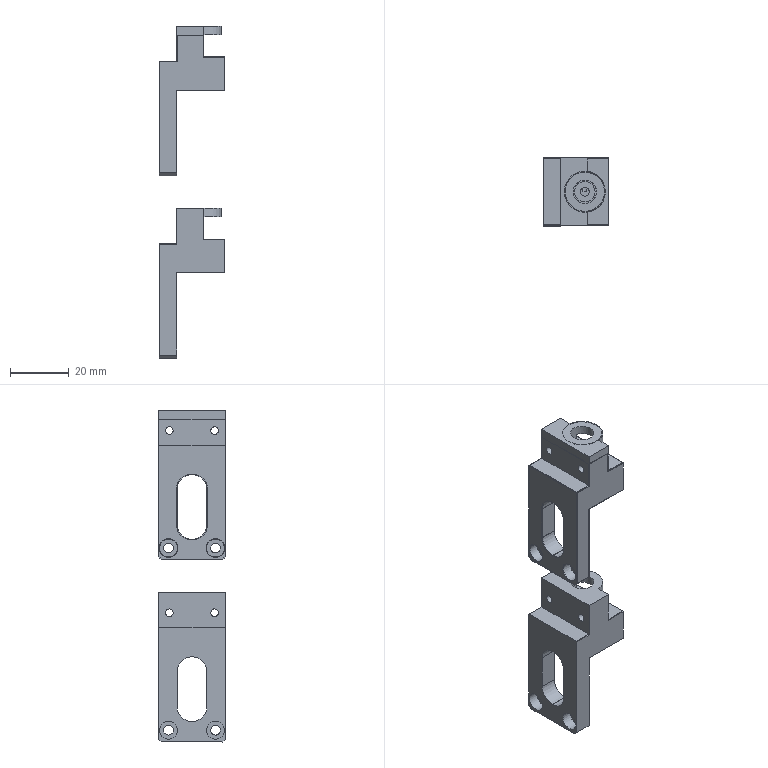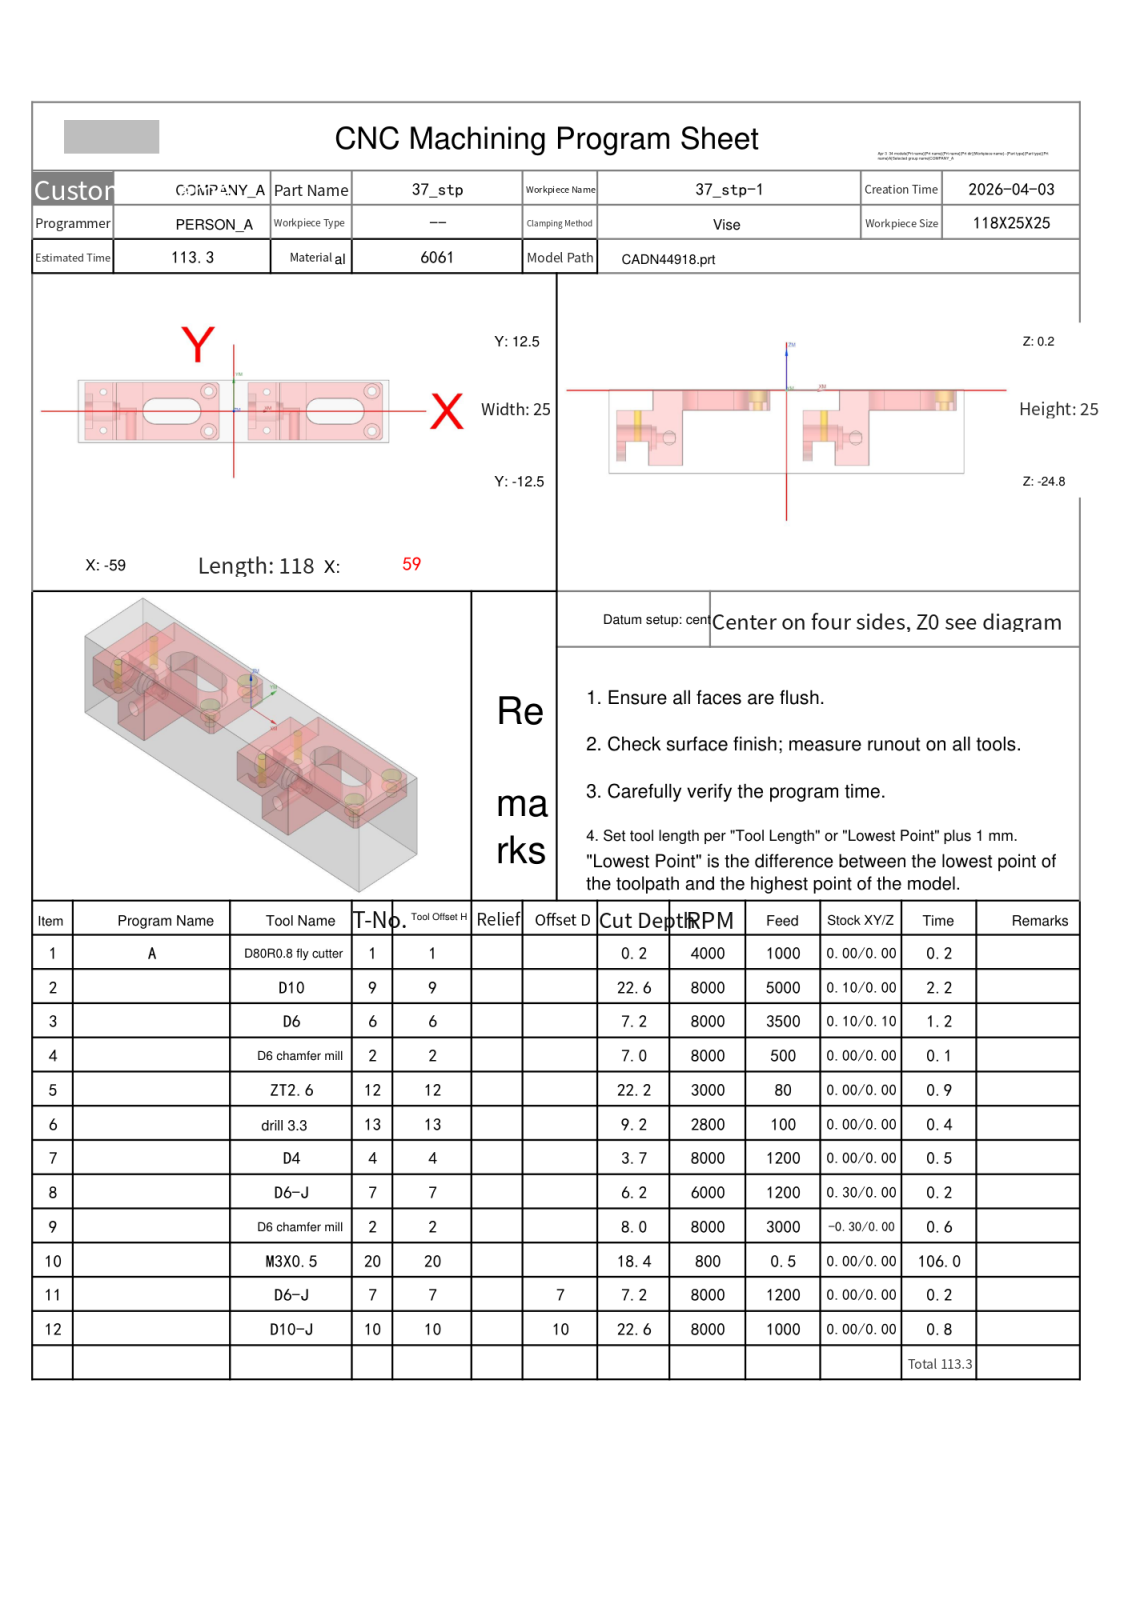NC program | NX | posted by the shop | part box 22.4 x 23 x 113 mm
Lines 1 to 2427 of 2531, first 1674 of 2425 lines:
%
O0001
(Machine time: 213.47 MIN)
(===Total Tool:10===)
(T1=D80R0.8 fly cutter D=80.  R=0.8  D-  H01 Z=0.    )
(T9=D10     D=10.  R=0.   D-  H09 Z=-22.4 )
(T6=D6      D=6.   R=0.   D-  H06 Z=-7.   )
(T2=D6 chamfer mill   D=6.   R=0.   D-  H02 Z=-7.8  )
(T12=ZT2.6  D=2.6  DR_a=118 D-  H12 Z=-22.  )
(T13=drill 3.3  D=3.3  DR_a=118 D-  H13 Z=-8.99 )
(T4=D4      D=4.   R=0.   D4  H04 Z=-3.5  )
(T7=D6-J    D=6.   R=0.   D-  H07 Z=-7.   )
(T20=M3X0.5 D=2.5  DR_a=180 D-  H20 Z=-18.25)
(T10=D10-J  D=10.  R=0.   D10 H10 Z=-22.4 )
G80 G90 G17 G49 G40
G91 G28 Z0
M01
N1 T01 M06
(D80R0.8 fly cutter  D=80. R=0.8 H=01 ce=0.00 di=0.00)
G00 G90 G54 X101.5 Y0.0 M03 S4000
G43 H01 Z20.
M08
Z2.
G01 Z0.0 F1000.
X96.5
X-96.5
X-101.5
Z2.
G00 Z20.
G91 G28 Z0.0
M05
M09
G91 G28 Z0.0
M01
N2 T09 M06
(D10  D=10. R=0. H=09 ce=0.10 di=0.00)
G00 G90 G54 X-31.5 Y-16.6 M03 S8000
G43 H09 Z20.
M08
Z.5
G01 X-56.5 Z.39 F5000.
G02 X-61.6 Y-11.5 Z.354 I0.0 J5.1
G01 Y11.5 Z.253
G02 X-56.5 Y16.6 Z.217 I5.1 J0.0
G01 X-45.75 Z.17
X-6.5 Z-.003
G02 X-2.894 Y15.106 Z-.021 I0.0 J-5.1
G01 X-1.894 Y14.106 Z-.027
G02 X-.4 Y10.5 Z-.045 I-3.606 J-3.606
G01 Y-10.5 Z-.138
G02 X-1.894 Y-14.106 Z-.155 I-5.1 J0.0
G01 X-2.894 Y-15.106 Z-.162
G02 X-6.5 Y-16.6 Z-.179 I-3.606 J3.606
G01 X-56.5 Z-.4
G02 X-61.6 Y-11.5 Z-.435 I0.0 J5.1
G01 Y11.5 Z-.537
G02 X-56.5 Y16.6 Z-.572 I5.1 J0.0
G01 X-45.75 Z-.62
X-6.5 Z-.793
G02 X-2.894 Y15.106 Z-.811 I0.0 J-5.1
G01 X-1.894 Y14.106 Z-.817
G02 X-.4 Y10.5 Z-.835 I-3.606 J-3.606
G01 Y-10.5 Z-.927
G02 X-1.894 Y-14.106 Z-.945 I-5.1 J0.0
G01 X-2.894 Y-15.106 Z-.951
G02 X-6.5 Y-16.6 Z-.969 I-3.606 J3.606
G01 X-56.5 Z-1.19
G02 X-61.6 Y-11.5 Z-1.225 I0.0 J5.1
G01 Y11.5 Z-1.327
G02 X-56.5 Y16.6 Z-1.362 I5.1 J0.0
G01 X-45.75 Z-1.409
X-6.5 Z-1.583
G02 X-2.894 Y15.106 Z-1.6 I0.0 J-5.1
G01 X-1.894 Y14.106 Z-1.607
G02 X-.4 Y10.5 Z-1.624 I-3.606 J-3.606
G01 Y-10.5 Z-1.717
G02 X-1.894 Y-14.106 Z-1.735 I-5.1 J0.0
G01 X-2.894 Y-15.106 Z-1.741
G02 X-6.5 Y-16.6 Z-1.759 I-3.606 J3.606
G01 X-56.5 Z-1.979
G02 X-61.6 Y-11.5 Z-2.015 I0.0 J5.1
G01 Y11.5 Z-2.116
G02 X-56.5 Y16.6 Z-2.152 I5.1 J0.0
G01 X-45.75 Z-2.199
X-6.5 Z-2.372
G02 X-2.894 Y15.106 Z-2.39 I0.0 J-5.1
G01 X-1.894 Y14.106 Z-2.396
G02 X-.4 Y10.5 Z-2.414 I-3.606 J-3.606
G01 Y-10.5 Z-2.507
G02 X-1.894 Y-14.106 Z-2.524 I-5.1 J0.0
G01 X-2.894 Y-15.106 Z-2.531
G02 X-6.5 Y-16.6 Z-2.548 I-3.606 J3.606
G01 X-56.5 Z-2.769
G02 X-61.6 Y-11.5 Z-2.804 I0.0 J5.1
G01 Y11.5 Z-2.906
G02 X-56.5 Y16.6 Z-2.941 I5.1 J0.0
G01 X-45.75 Z-2.989
X-6.5 Z-3.162
G02 X-2.894 Y15.106 Z-3.18 I0.0 J-5.1
G01 X-1.894 Y14.106 Z-3.186
G02 X-.4 Y10.5 Z-3.204 I-3.606 J-3.606
G01 Y-10.5 Z-3.296
G02 X-1.894 Y-14.106 Z-3.314 I-5.1 J0.0
G01 X-2.894 Y-15.106 Z-3.32
G02 X-6.5 Y-16.6 Z-3.338 I-3.606 J3.606
G01 X-56.5 Z-3.559
G02 X-61.6 Y-11.5 Z-3.594 I0.0 J5.1
G01 Y11.5 Z-3.696
G02 X-56.5 Y16.6 Z-3.731 I5.1 J0.0
G01 X-45.75 Z-3.778
X-6.5 Z-3.952
G02 X-2.894 Y15.106 Z-3.969 I0.0 J-5.1
G01 X-1.894 Y14.106 Z-3.976
G02 X-.4 Y10.5 Z-3.993 I-3.606 J-3.606
G01 Y-10.5 Z-4.086
G02 X-1.894 Y-14.106 Z-4.104 I-5.1 J0.0
G01 X-2.894 Y-15.106 Z-4.11
G02 X-6.5 Y-16.6 Z-4.128 I-3.606 J3.606
G01 X-56.5 Z-4.348
G02 X-61.6 Y-11.5 Z-4.384 I0.0 J5.1
G01 Y11.5 Z-4.485
G02 X-56.5 Y16.6 Z-4.521 I5.1 J0.0
G01 X-45.75 Z-4.568
X-6.5 Z-4.741
G02 X-2.894 Y15.106 Z-4.759 I0.0 J-5.1
G01 X-1.894 Y14.106 Z-4.765
G02 X-.4 Y10.5 Z-4.783 I-3.606 J-3.606
G01 Y-10.5 Z-4.876
G02 X-1.894 Y-14.106 Z-4.893 I-5.1 J0.0
G01 X-2.894 Y-15.106 Z-4.9
G02 X-6.5 Y-16.6 Z-4.917 I-3.606 J3.606
G01 X-56.5 Z-5.138
G02 X-61.6 Y-11.5 Z-5.173 I0.0 J5.1
G01 Y11.5 Z-5.275
G02 X-56.5 Y16.6 Z-5.31 I5.1 J0.0
G01 X-45.75 Z-5.358
X-6.5 Z-5.531
G02 X-2.894 Y15.106 Z-5.549 I0.0 J-5.1
G01 X-1.894 Y14.106 Z-5.555
G02 X-.4 Y10.5 Z-5.573 I-3.606 J-3.606
G01 Y-10.5 Z-5.665
G02 X-1.894 Y-14.106 Z-5.683 I-5.1 J0.0
G01 X-2.894 Y-15.106 Z-5.689
G02 X-6.5 Y-16.6 Z-5.707 I-3.606 J3.606
G01 X-56.5 Z-5.928
G02 X-61.6 Y-11.5 Z-5.963 I0.0 J5.1
G01 Y11.5 Z-6.065
G02 X-56.5 Y16.6 Z-6.1 I5.1 J0.0
G01 X-45.75 Z-6.147
X-6.5 Z-6.321
G02 X-2.894 Y15.106 Z-6.338 I0.0 J-5.1
G01 X-1.894 Y14.106 Z-6.345
G02 X-.4 Y10.5 Z-6.362 I-3.606 J-3.606
G01 Y-10.5 Z-6.455
G02 X-1.894 Y-14.106 Z-6.473 I-5.1 J0.0
G01 X-2.894 Y-15.106 Z-6.479
G02 X-6.5 Y-16.6 Z-6.497 I-3.606 J3.606
G01 X-56.5 Z-6.717
G02 X-61.6 Y-11.5 Z-6.753 I0.0 J5.1
G01 Y11.5 Z-6.854
G02 X-56.5 Y16.6 Z-6.89 I5.1 J0.0
G01 X-45.75 Z-6.937
X-6.5 Z-7.11
G02 X-2.894 Y15.106 Z-7.128 I0.0 J-5.1
G01 X-1.894 Y14.106 Z-7.134
G02 X-.4 Y10.5 Z-7.152 I-3.606 J-3.606
G01 Y-10.5 Z-7.245
G02 X-1.894 Y-14.106 Z-7.262 I-5.1 J0.0
G01 X-2.894 Y-15.106 Z-7.269
G02 X-6.5 Y-16.6 Z-7.286 I-3.606 J3.606
G01 X-56.5 Z-7.507
G02 X-61.6 Y-11.5 Z-7.542 I0.0 J5.1
G01 Y11.5 Z-7.644
G02 X-56.5 Y16.6 Z-7.679 I5.1 J0.0
G01 X-45.75 Z-7.727
X-6.5 Z-7.9
G02 X-2.894 Y15.106 Z-7.918 I0.0 J-5.1
G01 X-1.894 Y14.106 Z-7.924
G02 X-.4 Y10.5 Z-7.942 I-3.606 J-3.606
G01 Y-10.5 Z-8.034
G02 X-1.894 Y-14.106 Z-8.052 I-5.1 J0.0
G01 X-2.894 Y-15.106 Z-8.058
G02 X-6.5 Y-16.6 Z-8.076 I-3.606 J3.606
G01 X-56.5 Z-8.297
G02 X-61.6 Y-11.5 Z-8.332 I0.0 J5.1
G01 Y11.5 Z-8.433
G02 X-56.5 Y16.6 Z-8.469 I5.1 J0.0
G01 X-45.75 Z-8.516
X-6.5 Z-8.69
G02 X-2.894 Y15.106 Z-8.707 I0.0 J-5.1
G01 X-1.894 Y14.106 Z-8.713
G02 X-.4 Y10.5 Z-8.731 I-3.606 J-3.606
G01 Y-10.5 Z-8.824
G02 X-1.894 Y-14.106 Z-8.842 I-5.1 J0.0
G01 X-2.894 Y-15.106 Z-8.848
G02 X-6.5 Y-16.6 Z-8.865 I-3.606 J3.606
G01 X-56.5 Z-9.086
G02 X-61.6 Y-11.5 Z-9.122 I0.0 J5.1
G01 Y11.5 Z-9.223
G02 X-56.5 Y16.6 Z-9.258 I5.1 J0.0
G01 X-45.75 Z-9.306
X-6.5 Z-9.479
G02 X-2.894 Y15.106 Z-9.497 I0.0 J-5.1
G01 X-1.894 Y14.106 Z-9.503
G02 X-.4 Y10.5 Z-9.521 I-3.606 J-3.606
G01 Y-10.5 Z-9.614
G02 X-1.894 Y-14.106 Z-9.631 I-5.1 J0.0
G01 X-2.894 Y-15.106 Z-9.637
G02 X-6.5 Y-16.6 Z-9.655 I-3.606 J3.606
G01 X-56.5 Z-9.876
G02 X-61.6 Y-11.5 Z-9.911 I0.0 J5.1
G01 Y11.5 Z-10.013
G02 X-56.5 Y16.6 Z-10.048 I5.1 J0.0
G01 X-45.75 Z-10.096
X-6.5 Z-10.269
G02 X-2.894 Y15.106 Z-10.287 I0.0 J-5.1
G01 X-1.894 Y14.106 Z-10.293
G02 X-.4 Y10.5 Z-10.31 I-3.606 J-3.606
G01 Y-10.5 Z-10.403
G02 X-1.894 Y-14.106 Z-10.421 I-5.1 J0.0
G01 X-2.894 Y-15.106 Z-10.427
G02 X-6.5 Y-16.6 Z-10.445 I-3.606 J3.606
G01 X-56.5 Z-10.666
G02 X-61.6 Y-11.5 Z-10.701 I0.0 J5.1
G01 Y11.5 Z-10.802
G02 X-56.5 Y16.6 Z-10.838 I5.1 J0.0
G01 X-45.75 Z-10.885
X-6.5 Z-11.059
G02 X-2.894 Y15.106 Z-11.076 I0.0 J-5.1
G01 X-1.894 Y14.106 Z-11.082
G02 X-.4 Y10.5 Z-11.1 I-3.606 J-3.606
G01 Y-10.5 Z-11.193
G02 X-1.894 Y-14.106 Z-11.211 I-5.1 J0.0
G01 X-2.894 Y-15.106 Z-11.217
G02 X-6.5 Y-16.6 Z-11.234 I-3.606 J3.606
G01 X-56.5 Z-11.455
G02 X-61.6 Y-11.5 Z-11.491 I0.0 J5.1
G01 Y11.5 Z-11.592
G02 X-56.5 Y16.6 Z-11.627 I5.1 J0.0
G01 X-45.75 Z-11.675
X-6.5 Z-11.848
G02 X-2.894 Y15.106 Z-11.866 I0.0 J-5.1
G01 X-1.894 Y14.106 Z-11.872
G02 X-.4 Y10.5 Z-11.89 I-3.606 J-3.606
G01 Y-10.5 Z-11.983
G02 X-1.894 Y-14.106 Z-12. I-5.1 J0.0
G01 X-2.894 Y-15.106 Z-12.006
G02 X-6.5 Y-16.6 Z-12.024 I-3.606 J3.606
G01 X-56.5 Z-12.245
G02 X-61.6 Y-11.5 Z-12.28 I0.0 J5.1
G01 Y11.5 Z-12.382
G02 X-56.5 Y16.6 Z-12.417 I5.1 J0.0
G01 X-45.75 Z-12.465
X-6.5 Z-12.638
G02 X-2.894 Y15.106 Z-12.656 I0.0 J-5.1
G01 X-1.894 Y14.106 Z-12.662
G02 X-.4 Y10.5 Z-12.679 I-3.606 J-3.606
G01 Y-10.5 Z-12.772
G02 X-1.894 Y-14.106 Z-12.79 I-5.1 J0.0
G01 X-2.894 Y-15.106 Z-12.796
G02 X-6.5 Y-16.6 Z-12.814 I-3.606 J3.606
G01 X-56.5 Z-13.035
G02 X-61.6 Y-11.5 Z-13.07 I0.0 J5.1
G01 Y11.5 Z-13.171
G02 X-56.5 Y16.6 Z-13.207 I5.1 J0.0
G01 X-45.75 Z-13.254
X-6.5 Z-13.428
G02 X-2.894 Y15.106 Z-13.445 I0.0 J-5.1
G01 X-1.894 Y14.106 Z-13.451
G02 X-.4 Y10.5 Z-13.469 I-3.606 J-3.606
G01 Y-10.5 Z-13.562
G02 X-1.894 Y-14.106 Z-13.58 I-5.1 J0.0
G01 X-2.894 Y-15.106 Z-13.586
G02 X-6.5 Y-16.6 Z-13.603 I-3.606 J3.606
G01 X-56.5 Z-13.824
G02 X-61.6 Y-11.5 Z-13.86 I0.0 J5.1
G01 Y11.5 Z-13.961
G02 X-56.5 Y16.6 Z-13.996 I5.1 J0.0
G01 X-45.75 Z-14.044
X-6.5 Z-14.217
G02 X-2.894 Y15.106 Z-14.235 I0.0 J-5.1
G01 X-1.894 Y14.106 Z-14.241
G02 X-.4 Y10.5 Z-14.259 I-3.606 J-3.606
G01 Y-10.5 Z-14.351
G02 X-1.894 Y-14.106 Z-14.369 I-5.1 J0.0
G01 X-2.894 Y-15.106 Z-14.375
G02 X-6.5 Y-16.6 Z-14.393 I-3.606 J3.606
G01 X-56.5 Z-14.614
G02 X-61.6 Y-11.5 Z-14.649 I0.0 J5.1
G01 Y11.5 Z-14.751
G02 X-56.5 Y16.6 Z-14.786 I5.1 J0.0
G01 X-45.75 Z-14.834
X-6.5 Z-15.007
G02 X-2.894 Y15.106 Z-15.024 I0.0 J-5.1
G01 X-1.894 Y14.106 Z-15.031
G02 X-.4 Y10.5 Z-15.048 I-3.606 J-3.606
G01 Y-10.5 Z-15.141
G02 X-1.894 Y-14.106 Z-15.159 I-5.1 J0.0
G01 X-2.894 Y-15.106 Z-15.165
G02 X-6.5 Y-16.6 Z-15.183 I-3.606 J3.606
G01 X-56.5 Z-15.403
G02 X-61.6 Y-11.5 Z-15.439 I0.0 J5.1
G01 Y11.5 Z-15.54
G02 X-56.5 Y16.6 Z-15.576 I5.1 J0.0
G01 X-45.75 Z-15.623
X-6.5 Z-15.796
G02 X-2.894 Y15.106 Z-15.814 I0.0 J-5.1
G01 X-1.894 Y14.106 Z-15.82
G02 X-.4 Y10.5 Z-15.838 I-3.606 J-3.606
G01 Y-10.5 Z-15.931
G02 X-1.894 Y-14.106 Z-15.948 I-5.1 J0.0
G01 X-2.894 Y-15.106 Z-15.955
G02 X-6.5 Y-16.6 Z-15.972 I-3.606 J3.606
G01 X-56.5 Z-16.193
G02 X-61.6 Y-11.5 Z-16.228 I0.0 J5.1
G01 Y11.5 Z-16.33
G02 X-56.5 Y16.6 Z-16.365 I5.1 J0.0
G01 X-45.75 Z-16.413
X-6.5 Z-16.586
G02 X-2.894 Y15.106 Z-16.604 I0.0 J-5.1
G01 X-1.894 Y14.106 Z-16.61
G02 X-.4 Y10.5 Z-16.628 I-3.606 J-3.606
G01 Y-10.5 Z-16.72
G02 X-1.894 Y-14.106 Z-16.738 I-5.1 J0.0
G01 X-2.894 Y-15.106 Z-16.744
G02 X-6.5 Y-16.6 Z-16.762 I-3.606 J3.606
G01 X-56.5 Z-16.983
G02 X-61.6 Y-11.5 Z-17.018 I0.0 J5.1
G01 Y11.5 Z-17.12
G02 X-56.5 Y16.6 Z-17.155 I5.1 J0.0
G01 X-45.75 Z-17.203
X-6.5 Z-17.376
G02 X-2.894 Y15.106 Z-17.393 I0.0 J-5.1
G01 X-1.894 Y14.106 Z-17.4
G02 X-.4 Y10.5 Z-17.417 I-3.606 J-3.606
G01 Y-10.5 Z-17.51
G02 X-1.894 Y-14.106 Z-17.528 I-5.1 J0.0
G01 X-2.894 Y-15.106 Z-17.534
G02 X-6.5 Y-16.6 Z-17.552 I-3.606 J3.606
G01 X-56.5 Z-17.772
G02 X-61.6 Y-11.5 Z-17.808 I0.0 J5.1
G01 Y11.5 Z-17.909
G02 X-56.5 Y16.6 Z-17.945 I5.1 J0.0
G01 X-45.75 Z-17.992
X-6.5 Z-18.165
G02 X-2.894 Y15.106 Z-18.183 I0.0 J-5.1
G01 X-1.894 Y14.106 Z-18.189
G02 X-.4 Y10.5 Z-18.207 I-3.606 J-3.606
G01 Y-10.5 Z-18.3
G02 X-1.894 Y-14.106 Z-18.317 I-5.1 J0.0
G01 X-2.894 Y-15.106 Z-18.324
G02 X-6.5 Y-16.6 Z-18.341 I-3.606 J3.606
G01 X-56.5 Z-18.562
G02 X-61.6 Y-11.5 Z-18.597 I0.0 J5.1
G01 Y11.5 Z-18.699
G02 X-56.5 Y16.6 Z-18.734 I5.1 J0.0
G01 X-45.75 Z-18.782
X-6.5 Z-18.955
G02 X-2.894 Y15.106 Z-18.973 I0.0 J-5.1
G01 X-1.894 Y14.106 Z-18.979
G02 X-.4 Y10.5 Z-18.997 I-3.606 J-3.606
G01 Y-10.5 Z-19.089
G02 X-1.894 Y-14.106 Z-19.107 I-5.1 J0.0
G01 X-2.894 Y-15.106 Z-19.113
G02 X-6.5 Y-16.6 Z-19.131 I-3.606 J3.606
G01 X-56.5 Z-19.352
G02 X-61.6 Y-11.5 Z-19.387 I0.0 J5.1
G01 Y11.5 Z-19.489
G02 X-56.5 Y16.6 Z-19.524 I5.1 J0.0
G01 X-45.75 Z-19.571
X-6.5 Z-19.745
G02 X-2.894 Y15.106 Z-19.762 I0.0 J-5.1
G01 X-1.894 Y14.106 Z-19.769
G02 X-.4 Y10.5 Z-19.786 I-3.606 J-3.606
G01 Y-10.5 Z-19.879
G02 X-1.894 Y-14.106 Z-19.897 I-5.1 J0.0
G01 X-2.894 Y-15.106 Z-19.903
G02 X-6.5 Y-16.6 Z-19.921 I-3.606 J3.606
G01 X-56.5 Z-20.141
G02 X-61.6 Y-11.5 Z-20.177 I0.0 J5.1
G01 Y11.5 Z-20.278
G02 X-56.5 Y16.6 Z-20.314 I5.1 J0.0
G01 X-45.75 Z-20.361
X-6.5 Z-20.534
G02 X-2.894 Y15.106 Z-20.552 I0.0 J-5.1
G01 X-1.894 Y14.106 Z-20.558
G02 X-.4 Y10.5 Z-20.576 I-3.606 J-3.606
G01 Y-10.5 Z-20.669
G02 X-1.894 Y-14.106 Z-20.686 I-5.1 J0.0
G01 X-2.894 Y-15.106 Z-20.693
G02 X-6.5 Y-16.6 Z-20.71 I-3.606 J3.606
G01 X-56.5 Z-20.931
G02 X-61.6 Y-11.5 Z-20.966 I0.0 J5.1
G01 Y11.5 Z-21.068
G02 X-56.5 Y16.6 Z-21.103 I5.1 J0.0
G01 X-45.75 Z-21.151
X-6.5 Z-21.324
G02 X-2.894 Y15.106 Z-21.342 I0.0 J-5.1
G01 X-1.894 Y14.106 Z-21.348
G02 X-.4 Y10.5 Z-21.366 I-3.606 J-3.606
G01 Y-10.5 Z-21.458
G02 X-1.894 Y-14.106 Z-21.476 I-5.1 J0.0
G01 X-2.894 Y-15.106 Z-21.482
G02 X-6.5 Y-16.6 Z-21.5 I-3.606 J3.606
G01 X-56.5 Z-21.721
G02 X-61.6 Y-11.5 Z-21.756 I0.0 J5.1
G01 Y11.5 Z-21.858
G02 X-56.5 Y16.6 Z-21.893 I5.1 J0.0
G01 X-45.75 Z-21.94
X-6.5 Z-22.114
G02 X-2.894 Y15.106 Z-22.131 I0.0 J-5.1
G01 X-1.894 Y14.106 Z-22.138
G02 X-.4 Y10.5 Z-22.155 I-3.606 J-3.606
G01 Y-10.5 Z-22.248
G02 X-1.894 Y-14.106 Z-22.266 I-5.1 J0.0
G01 X-2.894 Y-15.106 Z-22.272
G02 X-6.5 Y-16.6 Z-22.29 I-3.606 J3.606
G01 X-31.5 Z-22.4
X-56.5
G02 X-61.6 Y-11.5 I0.0 J5.1
G01 Y11.5
G02 X-56.5 Y16.6 I5.1 J0.0
G01 X-45.75
X-6.5
G02 X-2.894 Y15.106 I0.0 J-5.1
G01 X-1.894 Y14.106
G02 X-.4 Y10.5 I-3.606 J-3.606
G01 Y-10.5
G02 X-1.894 Y-14.106 I-5.1 J0.0
G01 X-2.894 Y-15.106
G02 X-6.5 Y-16.6 I-3.606 J3.606
G01 X-31.5
X-32.
Z-21.4
G00 Z20.
X30.5
Z.5
G01 X5.5 Z.39
G02 X.4 Y-11.5 Z.354 I0.0 J5.1
G01 Y11.5 Z.253
G02 X3.44 Y16.165 Z.227 I5.1 J0.0
X5.5 Y16.6 Z.217 I2.06 J-4.665
G01 X55.5 Z-.003
G02 X59.106 Y15.106 Z-.021 I0.0 J-5.1
G01 X60.106 Y14.106 Z-.027
G02 X61.6 Y10.5 Z-.045 I-3.606 J-3.606
G01 Y-10.5 Z-.138
G02 X60.106 Y-14.106 Z-.155 I-5.1 J0.0
G01 X59.106 Y-15.106 Z-.162
G02 X55.5 Y-16.6 Z-.179 I-3.606 J3.606
G01 X5.5 Z-.4
G02 X.4 Y-11.5 Z-.435 I0.0 J5.1
G01 Y11.5 Z-.537
G02 X3.44 Y16.165 Z-.563 I5.1 J0.0
X5.5 Y16.6 Z-.572 I2.06 J-4.665
G01 X55.5 Z-.793
G02 X59.106 Y15.106 Z-.811 I0.0 J-5.1
G01 X60.106 Y14.106 Z-.817
G02 X61.6 Y10.5 Z-.835 I-3.606 J-3.606
G01 Y-10.5 Z-.927
G02 X60.106 Y-14.106 Z-.945 I-5.1 J0.0
G01 X59.106 Y-15.106 Z-.951
G02 X55.5 Y-16.6 Z-.969 I-3.606 J3.606
G01 X5.5 Z-1.19
G02 X.4 Y-11.5 Z-1.225 I0.0 J5.1
G01 Y11.5 Z-1.327
G02 X3.44 Y16.165 Z-1.353 I5.1 J0.0
X5.5 Y16.6 Z-1.362 I2.06 J-4.665
G01 X55.5 Z-1.583
G02 X59.106 Y15.106 Z-1.6 I0.0 J-5.1
G01 X60.106 Y14.106 Z-1.607
G02 X61.6 Y10.5 Z-1.624 I-3.606 J-3.606
G01 Y-10.5 Z-1.717
G02 X60.106 Y-14.106 Z-1.735 I-5.1 J0.0
G01 X59.106 Y-15.106 Z-1.741
G02 X55.5 Y-16.6 Z-1.759 I-3.606 J3.606
G01 X5.5 Z-1.979
G02 X.4 Y-11.5 Z-2.015 I0.0 J5.1
G01 Y11.5 Z-2.116
G02 X3.44 Y16.165 Z-2.142 I5.1 J0.0
X5.5 Y16.6 Z-2.152 I2.06 J-4.665
G01 X55.5 Z-2.372
G02 X59.106 Y15.106 Z-2.39 I0.0 J-5.1
G01 X60.106 Y14.106 Z-2.396
G02 X61.6 Y10.5 Z-2.414 I-3.606 J-3.606
G01 Y-10.5 Z-2.507
G02 X60.106 Y-14.106 Z-2.524 I-5.1 J0.0
G01 X59.106 Y-15.106 Z-2.531
G02 X55.5 Y-16.6 Z-2.548 I-3.606 J3.606
G01 X5.5 Z-2.769
G02 X.4 Y-11.5 Z-2.804 I0.0 J5.1
G01 Y11.5 Z-2.906
G02 X3.44 Y16.165 Z-2.932 I5.1 J0.0
X5.5 Y16.6 Z-2.941 I2.06 J-4.665
G01 X55.5 Z-3.162
G02 X59.106 Y15.106 Z-3.18 I0.0 J-5.1
G01 X60.106 Y14.106 Z-3.186
G02 X61.6 Y10.5 Z-3.204 I-3.606 J-3.606
G01 Y-10.5 Z-3.296
G02 X60.106 Y-14.106 Z-3.314 I-5.1 J0.0
G01 X59.106 Y-15.106 Z-3.32
G02 X55.5 Y-16.6 Z-3.338 I-3.606 J3.606
G01 X5.5 Z-3.559
G02 X.4 Y-11.5 Z-3.594 I0.0 J5.1
G01 Y11.5 Z-3.696
G02 X3.44 Y16.165 Z-3.722 I5.1 J0.0
X5.5 Y16.6 Z-3.731 I2.06 J-4.665
G01 X55.5 Z-3.952
G02 X59.106 Y15.106 Z-3.969 I0.0 J-5.1
G01 X60.106 Y14.106 Z-3.976
G02 X61.6 Y10.5 Z-3.993 I-3.606 J-3.606
G01 Y-10.5 Z-4.086
G02 X60.106 Y-14.106 Z-4.104 I-5.1 J0.0
G01 X59.106 Y-15.106 Z-4.11
G02 X55.5 Y-16.6 Z-4.128 I-3.606 J3.606
G01 X5.5 Z-4.348
G02 X.4 Y-11.5 Z-4.384 I0.0 J5.1
G01 Y11.5 Z-4.485
G02 X3.44 Y16.165 Z-4.511 I5.1 J0.0
X5.5 Y16.6 Z-4.521 I2.06 J-4.665
G01 X55.5 Z-4.741
G02 X59.106 Y15.106 Z-4.759 I0.0 J-5.1
G01 X60.106 Y14.106 Z-4.765
G02 X61.6 Y10.5 Z-4.783 I-3.606 J-3.606
G01 Y-10.5 Z-4.876
G02 X60.106 Y-14.106 Z-4.893 I-5.1 J0.0
G01 X59.106 Y-15.106 Z-4.9
G02 X55.5 Y-16.6 Z-4.917 I-3.606 J3.606
G01 X5.5 Z-5.138
G02 X.4 Y-11.5 Z-5.173 I0.0 J5.1
G01 Y11.5 Z-5.275
G02 X3.44 Y16.165 Z-5.301 I5.1 J0.0
X5.5 Y16.6 Z-5.31 I2.06 J-4.665
G01 X55.5 Z-5.531
G02 X59.106 Y15.106 Z-5.549 I0.0 J-5.1
G01 X60.106 Y14.106 Z-5.555
G02 X61.6 Y10.5 Z-5.573 I-3.606 J-3.606
G01 Y-10.5 Z-5.665
G02 X60.106 Y-14.106 Z-5.683 I-5.1 J0.0
G01 X59.106 Y-15.106 Z-5.689
G02 X55.5 Y-16.6 Z-5.707 I-3.606 J3.606
G01 X5.5 Z-5.928
G02 X.4 Y-11.5 Z-5.963 I0.0 J5.1
G01 Y11.5 Z-6.065
G02 X3.44 Y16.165 Z-6.091 I5.1 J0.0
X5.5 Y16.6 Z-6.1 I2.06 J-4.665
G01 X55.5 Z-6.321
G02 X59.106 Y15.106 Z-6.338 I0.0 J-5.1
G01 X60.106 Y14.106 Z-6.345
G02 X61.6 Y10.5 Z-6.362 I-3.606 J-3.606
G01 Y-10.5 Z-6.455
G02 X60.106 Y-14.106 Z-6.473 I-5.1 J0.0
G01 X59.106 Y-15.106 Z-6.479
G02 X55.5 Y-16.6 Z-6.497 I-3.606 J3.606
G01 X5.5 Z-6.717
G02 X.4 Y-11.5 Z-6.753 I0.0 J5.1
G01 Y11.5 Z-6.854
G02 X3.44 Y16.165 Z-6.88 I5.1 J0.0
X5.5 Y16.6 Z-6.89 I2.06 J-4.665
G01 X55.5 Z-7.11
G02 X59.106 Y15.106 Z-7.128 I0.0 J-5.1
G01 X60.106 Y14.106 Z-7.134
G02 X61.6 Y10.5 Z-7.152 I-3.606 J-3.606
G01 Y-10.5 Z-7.245
G02 X60.106 Y-14.106 Z-7.262 I-5.1 J0.0
G01 X59.106 Y-15.106 Z-7.269
G02 X55.5 Y-16.6 Z-7.286 I-3.606 J3.606
G01 X5.5 Z-7.507
G02 X.4 Y-11.5 Z-7.542 I0.0 J5.1
G01 Y11.5 Z-7.644
G02 X3.44 Y16.165 Z-7.67 I5.1 J0.0
X5.5 Y16.6 Z-7.679 I2.06 J-4.665
G01 X55.5 Z-7.9
G02 X59.106 Y15.106 Z-7.918 I0.0 J-5.1
G01 X60.106 Y14.106 Z-7.924
G02 X61.6 Y10.5 Z-7.942 I-3.606 J-3.606
G01 Y-10.5 Z-8.034
G02 X60.106 Y-14.106 Z-8.052 I-5.1 J0.0
G01 X59.106 Y-15.106 Z-8.058
G02 X55.5 Y-16.6 Z-8.076 I-3.606 J3.606
G01 X5.5 Z-8.297
G02 X.4 Y-11.5 Z-8.332 I0.0 J5.1
G01 Y11.5 Z-8.433
G02 X3.44 Y16.165 Z-8.459 I5.1 J0.0
X5.5 Y16.6 Z-8.469 I2.06 J-4.665
G01 X55.5 Z-8.69
G02 X59.106 Y15.106 Z-8.707 I0.0 J-5.1
G01 X60.106 Y14.106 Z-8.713
G02 X61.6 Y10.5 Z-8.731 I-3.606 J-3.606
G01 Y-10.5 Z-8.824
G02 X60.106 Y-14.106 Z-8.842 I-5.1 J0.0
G01 X59.106 Y-15.106 Z-8.848
G02 X55.5 Y-16.6 Z-8.865 I-3.606 J3.606
G01 X5.5 Z-9.086
G02 X.4 Y-11.5 Z-9.122 I0.0 J5.1
G01 Y11.5 Z-9.223
G02 X3.44 Y16.165 Z-9.249 I5.1 J0.0
X5.5 Y16.6 Z-9.258 I2.06 J-4.665
G01 X55.5 Z-9.479
G02 X59.106 Y15.106 Z-9.497 I0.0 J-5.1
G01 X60.106 Y14.106 Z-9.503
G02 X61.6 Y10.5 Z-9.521 I-3.606 J-3.606
G01 Y-10.5 Z-9.614
G02 X60.106 Y-14.106 Z-9.631 I-5.1 J0.0
G01 X59.106 Y-15.106 Z-9.637
G02 X55.5 Y-16.6 Z-9.655 I-3.606 J3.606
G01 X5.5 Z-9.876
G02 X.4 Y-11.5 Z-9.911 I0.0 J5.1
G01 Y11.5 Z-10.013
G02 X3.44 Y16.165 Z-10.039 I5.1 J0.0
X5.5 Y16.6 Z-10.048 I2.06 J-4.665
G01 X55.5 Z-10.269
G02 X59.106 Y15.106 Z-10.287 I0.0 J-5.1
G01 X60.106 Y14.106 Z-10.293
G02 X61.6 Y10.5 Z-10.31 I-3.606 J-3.606
G01 Y-10.5 Z-10.403
G02 X60.106 Y-14.106 Z-10.421 I-5.1 J0.0
G01 X59.106 Y-15.106 Z-10.427
G02 X55.5 Y-16.6 Z-10.445 I-3.606 J3.606
G01 X5.5 Z-10.666
G02 X.4 Y-11.5 Z-10.701 I0.0 J5.1
G01 Y11.5 Z-10.802
G02 X3.44 Y16.165 Z-10.828 I5.1 J0.0
X5.5 Y16.6 Z-10.838 I2.06 J-4.665
G01 X55.5 Z-11.059
G02 X59.106 Y15.106 Z-11.076 I0.0 J-5.1
G01 X60.106 Y14.106 Z-11.082
G02 X61.6 Y10.5 Z-11.1 I-3.606 J-3.606
G01 Y-10.5 Z-11.193
G02 X60.106 Y-14.106 Z-11.211 I-5.1 J0.0
G01 X59.106 Y-15.106 Z-11.217
G02 X55.5 Y-16.6 Z-11.234 I-3.606 J3.606
G01 X5.5 Z-11.455
G02 X.4 Y-11.5 Z-11.491 I0.0 J5.1
G01 Y11.5 Z-11.592
G02 X3.44 Y16.165 Z-11.618 I5.1 J0.0
X5.5 Y16.6 Z-11.627 I2.06 J-4.665
G01 X55.5 Z-11.848
G02 X59.106 Y15.106 Z-11.866 I0.0 J-5.1
G01 X60.106 Y14.106 Z-11.872
G02 X61.6 Y10.5 Z-11.89 I-3.606 J-3.606
G01 Y-10.5 Z-11.983
G02 X60.106 Y-14.106 Z-12. I-5.1 J0.0
G01 X59.106 Y-15.106 Z-12.006
G02 X55.5 Y-16.6 Z-12.024 I-3.606 J3.606
G01 X5.5 Z-12.245
G02 X.4 Y-11.5 Z-12.28 I0.0 J5.1
G01 Y11.5 Z-12.382
G02 X3.44 Y16.165 Z-12.408 I5.1 J0.0
X5.5 Y16.6 Z-12.417 I2.06 J-4.665
G01 X55.5 Z-12.638
G02 X59.106 Y15.106 Z-12.656 I0.0 J-5.1
G01 X60.106 Y14.106 Z-12.662
G02 X61.6 Y10.5 Z-12.679 I-3.606 J-3.606
G01 Y-10.5 Z-12.772
G02 X60.106 Y-14.106 Z-12.79 I-5.1 J0.0
G01 X59.106 Y-15.106 Z-12.796
G02 X55.5 Y-16.6 Z-12.814 I-3.606 J3.606
G01 X5.5 Z-13.035
G02 X.4 Y-11.5 Z-13.07 I0.0 J5.1
G01 Y11.5 Z-13.171
G02 X3.44 Y16.165 Z-13.197 I5.1 J0.0
X5.5 Y16.6 Z-13.207 I2.06 J-4.665
G01 X55.5 Z-13.428
G02 X59.106 Y15.106 Z-13.445 I0.0 J-5.1
G01 X60.106 Y14.106 Z-13.451
G02 X61.6 Y10.5 Z-13.469 I-3.606 J-3.606
G01 Y-10.5 Z-13.562
G02 X60.106 Y-14.106 Z-13.58 I-5.1 J0.0
G01 X59.106 Y-15.106 Z-13.586
G02 X55.5 Y-16.6 Z-13.603 I-3.606 J3.606
G01 X5.5 Z-13.824
G02 X.4 Y-11.5 Z-13.86 I0.0 J5.1
G01 Y11.5 Z-13.961
G02 X3.44 Y16.165 Z-13.987 I5.1 J0.0
X5.5 Y16.6 Z-13.996 I2.06 J-4.665
G01 X55.5 Z-14.217
G02 X59.106 Y15.106 Z-14.235 I0.0 J-5.1
G01 X60.106 Y14.106 Z-14.241
G02 X61.6 Y10.5 Z-14.259 I-3.606 J-3.606
G01 Y-10.5 Z-14.351
G02 X60.106 Y-14.106 Z-14.369 I-5.1 J0.0
G01 X59.106 Y-15.106 Z-14.375
G02 X55.5 Y-16.6 Z-14.393 I-3.606 J3.606
G01 X5.5 Z-14.614
G02 X.4 Y-11.5 Z-14.649 I0.0 J5.1
G01 Y11.5 Z-14.751
G02 X3.44 Y16.165 Z-14.777 I5.1 J0.0
X5.5 Y16.6 Z-14.786 I2.06 J-4.665
G01 X55.5 Z-15.007
G02 X59.106 Y15.106 Z-15.024 I0.0 J-5.1
G01 X60.106 Y14.106 Z-15.031
G02 X61.6 Y10.5 Z-15.048 I-3.606 J-3.606
G01 Y-10.5 Z-15.141
G02 X60.106 Y-14.106 Z-15.159 I-5.1 J0.0
G01 X59.106 Y-15.106 Z-15.165
G02 X55.5 Y-16.6 Z-15.183 I-3.606 J3.606
G01 X5.5 Z-15.403
G02 X.4 Y-11.5 Z-15.439 I0.0 J5.1
G01 Y11.5 Z-15.54
G02 X3.44 Y16.165 Z-15.566 I5.1 J0.0
X5.5 Y16.6 Z-15.576 I2.06 J-4.665
G01 X55.5 Z-15.796
G02 X59.106 Y15.106 Z-15.814 I0.0 J-5.1
G01 X60.106 Y14.106 Z-15.82
G02 X61.6 Y10.5 Z-15.838 I-3.606 J-3.606
G01 Y-10.5 Z-15.931
G02 X60.106 Y-14.106 Z-15.948 I-5.1 J0.0
G01 X59.106 Y-15.106 Z-15.955
G02 X55.5 Y-16.6 Z-15.972 I-3.606 J3.606
G01 X5.5 Z-16.193
G02 X.4 Y-11.5 Z-16.228 I0.0 J5.1
G01 Y11.5 Z-16.33
G02 X3.44 Y16.165 Z-16.356 I5.1 J0.0
X5.5 Y16.6 Z-16.365 I2.06 J-4.665
G01 X55.5 Z-16.586
G02 X59.106 Y15.106 Z-16.604 I0.0 J-5.1
G01 X60.106 Y14.106 Z-16.61
G02 X61.6 Y10.5 Z-16.628 I-3.606 J-3.606
G01 Y-10.5 Z-16.72
G02 X60.106 Y-14.106 Z-16.738 I-5.1 J0.0
G01 X59.106 Y-15.106 Z-16.744
G02 X55.5 Y-16.6 Z-16.762 I-3.606 J3.606
G01 X5.5 Z-16.983
G02 X.4 Y-11.5 Z-17.018 I0.0 J5.1
G01 Y11.5 Z-17.12
G02 X3.44 Y16.165 Z-17.146 I5.1 J0.0
X5.5 Y16.6 Z-17.155 I2.06 J-4.665
G01 X55.5 Z-17.376
G02 X59.106 Y15.106 Z-17.393 I0.0 J-5.1
G01 X60.106 Y14.106 Z-17.4
G02 X61.6 Y10.5 Z-17.417 I-3.606 J-3.606
G01 Y-10.5 Z-17.51
G02 X60.106 Y-14.106 Z-17.528 I-5.1 J0.0
G01 X59.106 Y-15.106 Z-17.534
G02 X55.5 Y-16.6 Z-17.552 I-3.606 J3.606
G01 X5.5 Z-17.772
G02 X.4 Y-11.5 Z-17.808 I0.0 J5.1
G01 Y11.5 Z-17.909
G02 X3.44 Y16.165 Z-17.935 I5.1 J0.0
X5.5 Y16.6 Z-17.945 I2.06 J-4.665
G01 X55.5 Z-18.165
G02 X59.106 Y15.106 Z-18.183 I0.0 J-5.1
G01 X60.106 Y14.106 Z-18.189
G02 X61.6 Y10.5 Z-18.207 I-3.606 J-3.606
G01 Y-10.5 Z-18.3
G02 X60.106 Y-14.106 Z-18.317 I-5.1 J0.0
G01 X59.106 Y-15.106 Z-18.324
G02 X55.5 Y-16.6 Z-18.341 I-3.606 J3.606
G01 X5.5 Z-18.562
G02 X.4 Y-11.5 Z-18.597 I0.0 J5.1
G01 Y11.5 Z-18.699
G02 X3.44 Y16.165 Z-18.725 I5.1 J0.0
X5.5 Y16.6 Z-18.734 I2.06 J-4.665
G01 X55.5 Z-18.955
G02 X59.106 Y15.106 Z-18.973 I0.0 J-5.1
G01 X60.106 Y14.106 Z-18.979
G02 X61.6 Y10.5 Z-18.997 I-3.606 J-3.606
G01 Y-10.5 Z-19.089
G02 X60.106 Y-14.106 Z-19.107 I-5.1 J0.0
G01 X59.106 Y-15.106 Z-19.113
G02 X55.5 Y-16.6 Z-19.131 I-3.606 J3.606
G01 X5.5 Z-19.352
G02 X.4 Y-11.5 Z-19.387 I0.0 J5.1
G01 Y11.5 Z-19.489
G02 X3.44 Y16.165 Z-19.515 I5.1 J0.0
X5.5 Y16.6 Z-19.524 I2.06 J-4.665
G01 X55.5 Z-19.745
G02 X59.106 Y15.106 Z-19.762 I0.0 J-5.1
G01 X60.106 Y14.106 Z-19.769
G02 X61.6 Y10.5 Z-19.786 I-3.606 J-3.606
G01 Y-10.5 Z-19.879
G02 X60.106 Y-14.106 Z-19.897 I-5.1 J0.0
G01 X59.106 Y-15.106 Z-19.903
G02 X55.5 Y-16.6 Z-19.921 I-3.606 J3.606
G01 X5.5 Z-20.141
G02 X.4 Y-11.5 Z-20.177 I0.0 J5.1
G01 Y11.5 Z-20.278
G02 X3.44 Y16.165 Z-20.304 I5.1 J0.0
X5.5 Y16.6 Z-20.314 I2.06 J-4.665
G01 X55.5 Z-20.534
G02 X59.106 Y15.106 Z-20.552 I0.0 J-5.1
G01 X60.106 Y14.106 Z-20.558
G02 X61.6 Y10.5 Z-20.576 I-3.606 J-3.606
G01 Y-10.5 Z-20.669
G02 X60.106 Y-14.106 Z-20.686 I-5.1 J0.0
G01 X59.106 Y-15.106 Z-20.693
G02 X55.5 Y-16.6 Z-20.71 I-3.606 J3.606
G01 X5.5 Z-20.931
G02 X.4 Y-11.5 Z-20.966 I0.0 J5.1
G01 Y11.5 Z-21.068
G02 X3.44 Y16.165 Z-21.094 I5.1 J0.0
X5.5 Y16.6 Z-21.103 I2.06 J-4.665
G01 X55.5 Z-21.324
G02 X59.106 Y15.106 Z-21.342 I0.0 J-5.1
G01 X60.106 Y14.106 Z-21.348
G02 X61.6 Y10.5 Z-21.366 I-3.606 J-3.606
G01 Y-10.5 Z-21.458
G02 X60.106 Y-14.106 Z-21.476 I-5.1 J0.0
G01 X59.106 Y-15.106 Z-21.482
G02 X55.5 Y-16.6 Z-21.5 I-3.606 J3.606
G01 X5.5 Z-21.721
G02 X.4 Y-11.5 Z-21.756 I0.0 J5.1
G01 Y11.5 Z-21.858
G02 X3.44 Y16.165 Z-21.884 I5.1 J0.0
X5.5 Y16.6 Z-21.893 I2.06 J-4.665
G01 X55.5 Z-22.114
G02 X59.106 Y15.106 Z-22.131 I0.0 J-5.1
G01 X60.106 Y14.106 Z-22.138
G02 X61.6 Y10.5 Z-22.155 I-3.606 J-3.606
G01 Y-10.5 Z-22.248
G02 X60.106 Y-14.106 Z-22.266 I-5.1 J0.0
G01 X59.106 Y-15.106 Z-22.272
G02 X55.5 Y-16.6 Z-22.29 I-3.606 J3.606
G01 X30.5 Z-22.4
X5.5
G02 X.4 Y-11.5 I0.0 J5.1
G01 Y11.5
G02 X5.5 Y16.6 I5.1 J0.0
G01 X55.5
G02 X59.106 Y15.106 I0.0 J-5.1
G01 X60.106 Y14.106
G02 X61.6 Y10.5 I-3.606 J-3.606
G01 Y-10.5
G02 X60.106 Y-14.106 I-5.1 J0.0
G01 X59.106 Y-15.106
G02 X55.5 Y-16.6 I-3.606 J3.606
G01 X30.5
X30.
Z-21.4
G00 Z20.
G91 G28 Z0.0
M05
M09
G91 G28 Z0.0
M01
N3 T06 M06
(D6  D=6. R=0. H=06 ce=0.10 di=0.10)
G00 G90 G54 X9.65 Y-17.5 M03 S6000
G43 H06 Z20.
M08
Z.008
G01 Z-.492 F3500.
Y-12.1
X4.9
Y12.1
X14.4
Y-12.1
X9.65
Y-7.9
X9.1
Y7.9
X10.2
Y-7.9
X9.65
X9.15
Z.008
G00 Z.5
X9.65 Y-17.5
Z-.483
G01 Z-.983
Y-12.1
X4.9
Y12.1
X14.4
Y-12.1
X9.65
Y-7.9
X9.1
Y7.9
X10.2
Y-7.9
X9.65
X9.15
Z-.483
G00 Z.008
X9.65 Y-17.5
Z-.975
G01 Z-1.475
Y-12.1
X4.9
Y12.1
X14.4
Y-12.1
X9.65
Y-7.9
X9.1
Y7.9
X10.2
Y-7.9
X9.65
X9.15
Z-.975
G00 Z-.483
X9.65 Y-17.5
Z-1.467
G01 Z-1.967
Y-12.1
X4.9
Y12.1
X14.4
Y-12.1
X9.65
Y-7.9
X9.1
Y7.9
X10.2
Y-7.9
X9.65
X9.15
Z-1.467
G00 Z-.975
X9.65 Y-17.5
Z-1.958
G01 Z-2.458
Y-12.1
X4.9
Y12.1
X14.4
Y-12.1
X9.65
Y-7.9
X9.1
Y7.9
X10.2
Y-7.9
X9.65
X9.15
Z-1.958
G00 Z-1.467
X9.65 Y-17.5
Z-2.45
G01 Z-2.95
Y-12.1
X4.9
Y12.1
X14.4
Y-12.1
X9.65
Y-7.9
X9.1
Y7.9
X10.2
Y-7.9
X9.65
X9.15
Z-2.45
G00 Z-1.958
X9.65 Y-17.5
Z-2.942
G01 Z-3.442
Y-12.1
X4.9
Y12.1
X14.4
Y-12.1
X9.65
Y-7.9
X9.1
Y7.9
X10.2
Y-7.9
X9.65
X9.15
Z-2.942
G00 Z-2.45
X9.65 Y-17.5
Z-3.433
G01 Z-3.933
Y-12.1
X4.9
Y12.1
X14.4
Y-12.1
X9.65
Y-7.9
X9.1
Y7.9
X10.2
Y-7.9
X9.65
X9.15
Z-3.433
G00 Z-2.942
X9.65 Y-17.5
Z-3.925
G01 Z-4.425
Y-12.1
X4.9
Y12.1
X14.4
Y-12.1
X9.65
Y-7.9
X9.1
Y7.9
X10.2
Y-7.9
X9.65
X9.15
Z-3.925
G00 Z-3.433
X9.65 Y-17.5
Z-4.417
G01 Z-4.917
Y-12.1
X4.9
Y12.1
X14.4
Y-12.1
X9.65
Y-7.9
X9.1
Y7.9
X10.2
Y-7.9
X9.65
X9.15
Z-4.417
G00 Z-3.925
X9.65 Y-17.5
Z-4.908
G01 Z-5.408
Y-12.1
X4.9
Y12.1
X14.4
Y-12.1
X9.65
Y-7.9
X9.1
Y7.9
X10.2
Y-7.9
X9.65
X9.15
Z-4.908
G00 Z-4.417
X9.65 Y-17.5
Z-5.4
G01 Z-5.9
Y-12.1
X4.9
Y12.1
X14.4
Y-12.1
X9.65
Y-7.9
X9.1
Y7.9
X10.2
Y-7.9
X9.65
X9.15
Z-5.4
G00 Z20.
X-62.5 Y0.0
Z.008
G01 Z-.492
X-57.1
Y12.1
X-47.6
Y-12.1
X-57.1
Y0.0
X-52.9
Y7.9
X-51.8
Y-7.9
X-52.9
Y0.0
Y.5
Z.008
G00 Z.5
X-62.5 Y0.0
Z-.483
G01 Z-.983
X-57.1
Y12.1
X-47.6
Y-12.1
X-57.1
Y0.0
X-52.9
Y7.9
X-51.8
Y-7.9
X-52.9
Y0.0
Y.5
Z-.483
G00 Z.008
X-62.5 Y0.0
Z-.975
G01 Z-1.475
X-57.1
Y12.1
X-47.6
Y-12.1
X-57.1
Y0.0
X-52.9
Y7.9
X-51.8
Y-7.9
X-52.9
Y0.0
Y.5
Z-.975
G00 Z-.483
X-62.5 Y0.0
Z-1.467
G01 Z-1.967
X-57.1
Y12.1
X-47.6
Y-12.1
X-57.1
Y0.0
X-52.9
Y7.9
X-51.8
Y-7.9
X-52.9
Y0.0
Y.5
Z-1.467
G00 Z-.975
X-62.5 Y0.0
Z-1.958
G01 Z-2.458
X-57.1
Y12.1
X-47.6
Y-12.1
X-57.1
Y0.0
X-52.9
Y7.9
X-51.8
Y-7.9
X-52.9
Y0.0
Y.5
Z-1.958
G00 Z-1.467
X-62.5 Y0.0
Z-2.45
G01 Z-2.95
X-57.1
Y12.1
X-47.6
Y-12.1
X-57.1
Y0.0
X-52.9
Y7.9
X-51.8
Y-7.9
X-52.9
Y0.0
Y.5
Z-2.45
G00 Z-1.958
X-62.5 Y0.0
Z-2.942
G01 Z-3.442
X-57.1
Y12.1
X-47.6
Y-12.1
X-57.1
Y0.0
X-52.9
Y7.9
X-51.8
Y-7.9
X-52.9
Y0.0
Y.5
Z-2.942
G00 Z-2.45
X-62.5 Y0.0
Z-3.433
G01 Z-3.933
X-57.1
Y12.1
X-47.6
Y-12.1
X-57.1
Y0.0
X-52.9
Y7.9
X-51.8
Y-7.9
X-52.9
Y0.0
Y.5
Z-3.433
G00 Z-2.942
X-62.5 Y0.0
Z-3.925
G01 Z-4.425
X-57.1
Y12.1
X-47.6
Y-12.1
X-57.1
Y0.0
X-52.9
Y7.9
X-51.8
Y-7.9
X-52.9
Y0.0
Y.5
Z-3.925
G00 Z-3.433
X-62.5 Y0.0
Z-4.417
G01 Z-4.917
X-57.1
Y12.1
X-47.6
Y-12.1
X-57.1
Y0.0
X-52.9
Y7.9
X-51.8
Y-7.9
X-52.9
Y0.0
Y.5
Z-4.417
G00 Z-3.925
X-62.5 Y0.0
Z-4.908
G01 Z-5.408
X-57.1
Y12.1
X-47.6
Y-12.1
X-57.1
Y0.0
X-52.9
Y7.9
X-51.8
Y-7.9
X-52.9
Y0.0
Y.5
Z-4.908
G00 Z-4.417
X-62.5 Y0.0
Z-5.4
G01 Z-5.9
X-57.1
Y12.1
X-47.6
Y-12.1
X-57.1
Y0.0
X-52.9
Y7.9
X-51.8
Y-7.9
X-52.9
Y0.0
Y.5
Z-5.4
G00 Z20.
G00 G90 X-25.333 Y2. M03 S8000
Z20.
Z1.
G01 X-29.506 Z.781 F3000.
X-29.845 Y1.999 Z.764
X-30.567 Y1.708 Z.723
X-31.116 Y1.156 Z.682
X-31.401 Y.432 Z.641
X-31.4 Y.093 Z.623
Y-.1 Z.613
Y-.439 Z.596
X-31.112 Y-1.162 Z.555
X-30.561 Y-1.712 Z.514
X-29.839 Y-2. Z.473
X-29.5 Z.455
X-17.502 Z-.173
X-17.163 Z-.191
X-16.438 Y-1.711 Z-.232
X-15.886 Y-1.158 Z-.273
X-15.599 Y-.432 Z-.314
X-15.6 Y-.093 Z-.332
Y.1 Z-.342
Y.439 Z-.36
X-15.889 Y1.164 Z-.4
X-16.442 Y1.714 Z-.441
X-17.168 Y2.001 Z-.482
X-17.507 Y2. Z-.5
X-29.506
G03 X-31.4 Y.1 I.006 J-1.9
G01 Y.093
Y-.1
G03 X-29.5 Y-2. I1.9 J0.0
G01 X-17.502
X-17.5
G03 X-15.6 Y-.1 I0.0 J1.9
G01 Y-.093
Y.1
G03 X-17.5 Y2. I-1.9 J0.0
G01 X-17.507
X-27.048 Z-1.
X-29.506
G03 X-31.4 Y.1 I.006 J-1.9
G01 Y.093
Y-.1
G03 X-29.5 Y-2. I1.9 J0.0
G01 X-17.502
X-17.5
G03 X-15.6 Y-.1 I0.0 J1.9
G01 Y-.093
Y.1
G03 X-17.5 Y2. I-1.9 J0.0
G01 X-17.507
X-27.048 Z-1.5
X-29.506
G03 X-31.4 Y.1 I.006 J-1.9
G01 Y.093
Y-.1
G03 X-29.5 Y-2. I1.9 J0.0
G01 X-17.502
X-17.5
G03 X-15.6 Y-.1 I0.0 J1.9
G01 Y-.093
Y.1
G03 X-17.5 Y2. I-1.9 J0.0
G01 X-17.507
X-27.048 Z-2.
X-29.506
G03 X-31.4 Y.1 I.006 J-1.9
G01 Y.093
Y-.1
G03 X-29.5 Y-2. I1.9 J0.0
G01 X-17.502
X-17.5
G03 X-15.6 Y-.1 I0.0 J1.9
G01 Y-.093
Y.1
G03 X-17.5 Y2. I-1.9 J0.0
G01 X-17.507
X-27.048 Z-2.5
X-29.506
G03 X-31.4 Y.1 I.006 J-1.9
G01 Y.093
Y-.1
G03 X-29.5 Y-2. I1.9 J0.0
G01 X-17.502
X-17.5
G03 X-15.6 Y-.1 I0.0 J1.9
G01 Y-.093
Y.1
G03 X-17.5 Y2. I-1.9 J0.0
G01 X-17.507
X-27.048 Z-3.
X-29.506
G03 X-31.4 Y.1 I.006 J-1.9
G01 Y.093
Y-.1
G03 X-29.5 Y-2. I1.9 J0.0
G01 X-17.502
X-17.5
G03 X-15.6 Y-.1 I0.0 J1.9
G01 Y-.093
Y.1
G03 X-17.5 Y2. I-1.9 J0.0
G01 X-17.507
X-27.048 Z-3.5
X-29.506
G03 X-31.4 Y.1 I.006 J-1.9
G01 Y.093
Y-.1
G03 X-29.5 Y-2. I1.9 J0.0
G01 X-17.502
X-17.5
G03 X-15.6 Y-.1 I0.0 J1.9
G01 Y-.093
Y.1
G03 X-17.5 Y2. I-1.9 J0.0
G01 X-17.507
X-27.048 Z-4.
X-29.506
G03 X-31.4 Y.1 I.006 J-1.9
G01 Y.093
Y-.1
G03 X-29.5 Y-2. I1.9 J0.0
G01 X-17.502
X-17.5
G03 X-15.6 Y-.1 I0.0 J1.9
G01 Y-.093
Y.1
G03 X-17.5 Y2. I-1.9 J0.0
G01 X-17.507
X-27.048 Z-4.5
X-29.506
G03 X-31.4 Y.1 I.006 J-1.9
G01 Y.093
Y-.1
G03 X-29.5 Y-2. I1.9 J0.0
G01 X-17.502
X-17.5
G03 X-15.6 Y-.1 I0.0 J1.9
G01 Y-.093
Y.1
G03 X-17.5 Y2. I-1.9 J0.0
G01 X-17.507
X-27.048 Z-5.
X-29.506
G03 X-31.4 Y.1 I.006 J-1.9
G01 Y.093
Y-.1
G03 X-29.5 Y-2. I1.9 J0.0
G01 X-17.502
X-17.5
G03 X-15.6 Y-.1 I0.0 J1.9
G01 Y-.093
Y.1
G03 X-17.5 Y2. I-1.9 J0.0
G01 X-17.507
X-27.048 Z-5.5
X-29.506
G03 X-31.4 Y.1 I.006 J-1.9
G01 Y.093
Y-.1
G03 X-29.5 Y-2. I1.9 J0.0
G01 X-17.502
X-17.5
G03 X-15.6 Y-.1 I0.0 J1.9
G01 Y-.093
Y.1
G03 X-17.5 Y2. I-1.9 J0.0
G01 X-17.507
X-27.048 Z-6.
X-29.506
G03 X-31.4 Y.1 I.006 J-1.9
G01 Y.093
Y-.1
G03 X-29.5 Y-2. I1.9 J0.0
G01 X-17.502
X-17.5
G03 X-15.6 Y-.1 I0.0 J1.9
G01 Y-.093
Y.1
G03 X-17.5 Y2. I-1.9 J0.0
G01 X-17.507
X-27.048 Z-6.5
X-29.506
G03 X-31.4 Y.1 I.006 J-1.9
G01 Y.093
Y-.1
G03 X-29.5 Y-2. I1.9 J0.0
G01 X-17.502
X-17.5
G03 X-15.6 Y-.1 I0.0 J1.9
G01 Y-.093
Y.1
G03 X-17.5 Y2. I-1.9 J0.0
G01 X-17.507
X-27.048 Z-7.
X-29.506
G03 X-31.4 Y.1 I.006 J-1.9
G01 Y.093
Y-.1
G03 X-29.5 Y-2. I1.9 J0.0
G01 X-17.502
X-17.5
G03 X-15.6 Y-.1 I0.0 J1.9
G01 Y-.093
Y.1
G03 X-17.5 Y2. I-1.9 J0.0
G01 X-17.507
X-27.048
Z-6.
G00 Z20.
X36.667
Z1.
G01 X32.494 Z.781
X32.155 Y1.999 Z.764
X31.433 Y1.708 Z.723
X30.884 Y1.156 Z.682
X30.599 Y.432 Z.641
X30.6 Y.093 Z.623
Y-.1 Z.613
Y-.439 Z.596
X30.888 Y-1.162 Z.555
X31.439 Y-1.712 Z.514
X32.161 Y-2. Z.473
X32.5 Z.455
X44.498 Z-.173
X44.837 Z-.191
X45.563 Y-1.711 Z-.232
X46.114 Y-1.158 Z-.273
X46.401 Y-.432 Z-.314
X46.4 Y-.093 Z-.332
Y.1 Z-.342
Y.439 Z-.36
X46.111 Y1.163 Z-.4
X45.558 Y1.714 Z-.441
X44.832 Y2.001 Z-.482
X44.493 Y2. Z-.5
X32.494
G03 X30.6 Y.1 I.006 J-1.9
G01 Y.093
Y-.1
G03 X32.5 Y-2. I1.9 J0.0
G01 X44.498
X44.5
G03 X46.4 Y-.1 I0.0 J1.9
G01 Y-.093
Y.1
G03 X44.5 Y2. I-1.9 J0.0
G01 X44.493
X34.952 Z-1.
X32.494
G03 X30.6 Y.1 I.006 J-1.9
G01 Y.093
Y-.1
G03 X32.5 Y-2. I1.9 J0.0
G01 X44.498
X44.5
G03 X46.4 Y-.1 I0.0 J1.9
G01 Y-.093
Y.1
G03 X44.5 Y2. I-1.9 J0.0
G01 X44.493
X34.952 Z-1.5
X32.494
G03 X30.6 Y.1 I.006 J-1.9
G01 Y.093
Y-.1
G03 X32.5 Y-2. I1.9 J0.0
G01 X44.498
X44.5
G03 X46.4 Y-.1 I0.0 J1.9
G01 Y-.093
Y.1
G03 X44.5 Y2. I-1.9 J0.0
G01 X44.493
X34.952 Z-2.
X32.494
G03 X30.6 Y.1 I.006 J-1.9
G01 Y.093
Y-.1
G03 X32.5 Y-2. I1.9 J0.0
G01 X44.498
X44.5
G03 X46.4 Y-.1 I0.0 J1.9
G01 Y-.093
Y.1
G03 X44.5 Y2. I-1.9 J0.0
G01 X44.493
X34.952 Z-2.5
X32.494
G03 X30.6 Y.1 I.006 J-1.9
G01 Y.093
Y-.1
G03 X32.5 Y-2. I1.9 J0.0
G01 X44.498
X44.5
G03 X46.4 Y-.1 I0.0 J1.9
G01 Y-.093
Y.1
G03 X44.5 Y2. I-1.9 J0.0
G01 X44.493
X34.952 Z-3.
X32.494
G03 X30.6 Y.1 I.006 J-1.9
G01 Y.093
Y-.1
G03 X32.5 Y-2. I1.9 J0.0
G01 X44.498
X44.5
G03 X46.4 Y-.1 I0.0 J1.9
G01 Y-.093
Y.1
G03 X44.5 Y2. I-1.9 J0.0
G01 X44.493
X34.952 Z-3.5
X32.494
G03 X30.6 Y.1 I.006 J-1.9
G01 Y.093
Y-.1
G03 X32.5 Y-2. I1.9 J0.0
G01 X44.498
X44.5
G03 X46.4 Y-.1 I0.0 J1.9
G01 Y-.093
Y.1
G03 X44.5 Y2. I-1.9 J0.0
G01 X44.493
X34.952 Z-4.
X32.494
G03 X30.6 Y.1 I.006 J-1.9
G01 Y.093
Y-.1
G03 X32.5 Y-2. I1.9 J0.0
G01 X44.498
X44.5
G03 X46.4 Y-.1 I0.0 J1.9
G01 Y-.093
Y.1
G03 X44.5 Y2. I-1.9 J0.0
G01 X44.493
X34.952 Z-4.5
X32.494
G03 X30.6 Y.1 I.006 J-1.9
G01 Y.093
Y-.1
G03 X32.5 Y-2. I1.9 J0.0
G01 X44.498
X44.5
G03 X46.4 Y-.1 I0.0 J1.9
G01 Y-.093
Y.1
G03 X44.5 Y2. I-1.9 J0.0
G01 X44.493
X34.952 Z-5.
X32.494
G03 X30.6 Y.1 I.006 J-1.9
G01 Y.093
Y-.1
G03 X32.5 Y-2. I1.9 J0.0
G01 X44.498
X44.5
G03 X46.4 Y-.1 I0.0 J1.9
G01 Y-.093
Y.1
G03 X44.5 Y2. I-1.9 J0.0
G01 X44.493
X34.952 Z-5.5
X32.494
G03 X30.6 Y.1 I.006 J-1.9
G01 Y.093
Y-.1
G03 X32.5 Y-2. I1.9 J0.0
G01 X44.498
X44.5
G03 X46.4 Y-.1 I0.0 J1.9
G01 Y-.093
Y.1
G03 X44.5 Y2. I-1.9 J0.0
G01 X44.493
X34.952 Z-6.
X32.494
G03 X30.6 Y.1 I.006 J-1.9
G01 Y.093
Y-.1
G03 X32.5 Y-2. I1.9 J0.0
G01 X44.498
X44.5
G03 X46.4 Y-.1 I0.0 J1.9
G01 Y-.093
Y.1
G03 X44.5 Y2. I-1.9 J0.0
G01 X44.493
X34.952 Z-6.5
X32.494
G03 X30.6 Y.1 I.006 J-1.9
G01 Y.093
Y-.1
G03 X32.5 Y-2. I1.9 J0.0
G01 X44.498
X44.5
G03 X46.4 Y-.1 I0.0 J1.9
G01 Y-.093